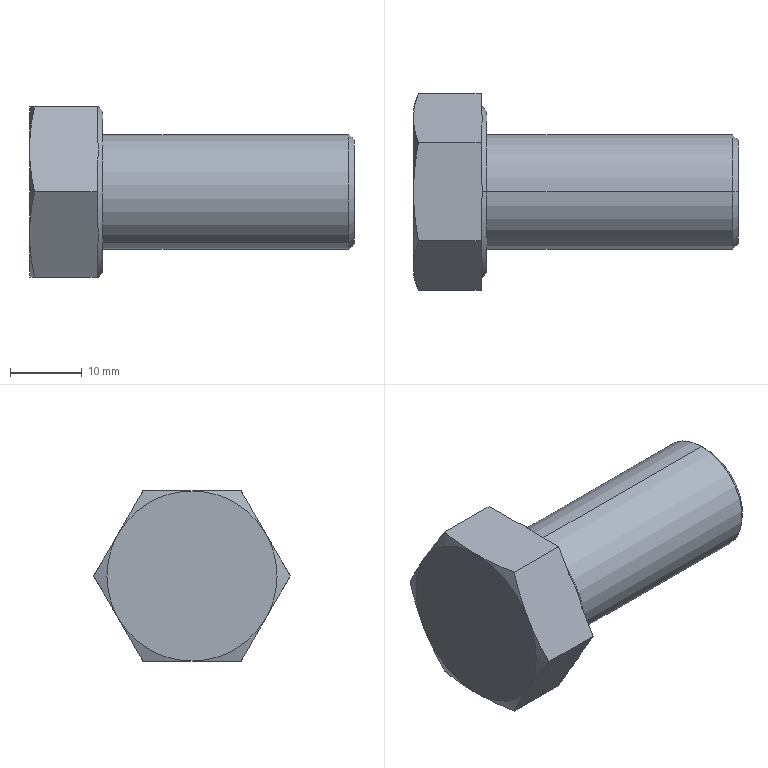Part | SolidWorks | 1 solid | 27 faces | box 45.18 x 27.332 x 23.67 mm | volume 11904 mm3 | plane 15 | cone 10 | cylinder 2 | commonest cylinder face diameters 16 x2
STEP:
#1=CARTESIAN_POINT('',(45.18,0.,-7.2));
#2=VERTEX_POINT('',#1);
#3=CARTESIAN_POINT('',(45.18,0.,7.2));
#4=VERTEX_POINT('',#3);
#5=CARTESIAN_POINT('',(45.18,0.,0.));
#6=DIRECTION('',(1.,0.,0.));
#7=DIRECTION('',(0.,0.,-1.));
#8=AXIS2_PLACEMENT_3D('',#5,#6,#7);
#9=CIRCLE('',#8,7.2);
#10=EDGE_CURVE('',#2,#4,#9,.T.);
#11=ORIENTED_EDGE('',*,*,#10,.F.);
#12=CARTESIAN_POINT('',(44.38,0.,-8.));
#13=VERTEX_POINT('',#12);
#14=CARTESIAN_POINT('',(45.18,0.,-7.2));
#15=DIRECTION('',(-0.7071,0.,-0.7071));
#16=VECTOR('',#15,1000.);
#17=LINE('',#14,#16);
#18=EDGE_CURVE('',#2,#13,#17,.T.);
#19=ORIENTED_EDGE('',*,*,#18,.T.);
#20=CARTESIAN_POINT('',(44.38,0.,8.));
#21=VERTEX_POINT('',#20);
#22=CARTESIAN_POINT('',(44.38,0.,0.));
#23=DIRECTION('',(-1.,0.,0.));
#24=DIRECTION('',(0.,0.,-1.));
#25=AXIS2_PLACEMENT_3D('',#22,#23,#24);
#26=CIRCLE('',#25,8.);
#27=EDGE_CURVE('',#21,#13,#26,.T.);
#28=ORIENTED_EDGE('',*,*,#27,.F.);
#29=CARTESIAN_POINT('',(45.18,0.,7.2));
#30=DIRECTION('',(-0.7071,0.,0.7071));
#31=VECTOR('',#30,1000.);
#32=LINE('',#29,#31);
#33=EDGE_CURVE('',#4,#21,#32,.T.);
#34=ORIENTED_EDGE('',*,*,#33,.F.);
#35=EDGE_LOOP('',(#11,#19,#28,#34));
#36=FACE_OUTER_BOUND('',#35,.T.);
#37=CARTESIAN_POINT('',(45.18,0.,0.));
#38=DIRECTION('',(-1.,0.,0.));
#39=DIRECTION('',(0.,0.,1.));
#40=AXIS2_PLACEMENT_3D('',#37,#38,#39);
#41=CONICAL_SURFACE('',#40,7.2,0.7854);
#42=ADVANCED_FACE('',(#36),#41,.T.);
#43=ORIENTED_EDGE('',*,*,#27,.T.);
#44=CARTESIAN_POINT('',(10.18,0.,-8.));
#45=VERTEX_POINT('',#44);
#46=CARTESIAN_POINT('',(45.18,0.,-8.));
#47=DIRECTION('',(-1.,0.,0.));
#48=VECTOR('',#47,1000.);
#49=LINE('',#46,#48);
#50=EDGE_CURVE('',#13,#45,#49,.T.);
#51=ORIENTED_EDGE('',*,*,#50,.T.);
#52=CARTESIAN_POINT('',(10.18,0.,8.));
#53=VERTEX_POINT('',#52);
#54=CARTESIAN_POINT('',(10.18,0.,0.));
#55=DIRECTION('',(1.,0.,0.));
#56=DIRECTION('',(0.,0.,1.));
#57=AXIS2_PLACEMENT_3D('',#54,#55,#56);
#58=CIRCLE('',#57,8.);
#59=EDGE_CURVE('',#45,#53,#58,.T.);
#60=ORIENTED_EDGE('',*,*,#59,.T.);
#61=CARTESIAN_POINT('',(45.18,0.,8.));
#62=DIRECTION('',(-1.,0.,0.));
#63=VECTOR('',#62,1000.);
#64=LINE('',#61,#63);
#65=EDGE_CURVE('',#21,#53,#64,.T.);
#66=ORIENTED_EDGE('',*,*,#65,.F.);
#67=EDGE_LOOP('',(#43,#51,#60,#66));
#68=FACE_OUTER_BOUND('',#67,.T.);
#69=CARTESIAN_POINT('',(45.18,0.,0.));
#70=DIRECTION('',(-1.,0.,0.));
#71=DIRECTION('',(0.,0.,1.));
#72=AXIS2_PLACEMENT_3D('',#69,#70,#71);
#73=CYLINDRICAL_SURFACE('',#72,8.);
#74=ADVANCED_FACE('',(#68),#73,.T.);
#75=CARTESIAN_POINT('',(10.18,0.,11.245));
#76=VERTEX_POINT('',#75);
#77=CARTESIAN_POINT('',(10.18,0.,-11.245));
#78=VERTEX_POINT('',#77);
#79=CARTESIAN_POINT('',(10.18,0.,0.));
#80=DIRECTION('',(-1.,0.,0.));
#81=DIRECTION('',(0.,0.,1.));
#82=AXIS2_PLACEMENT_3D('',#79,#80,#81);
#83=CIRCLE('',#82,11.245);
#84=EDGE_CURVE('',#76,#78,#83,.T.);
#85=ORIENTED_EDGE('',*,*,#84,.T.);
#86=CARTESIAN_POINT('',(9.59,0.,-11.835));
#87=VERTEX_POINT('',#86);
#88=CARTESIAN_POINT('',(9.38,0.,-12.045));
#89=DIRECTION('',(-0.7071,0.,-0.7071));
#90=VECTOR('',#89,1000.);
#91=LINE('',#88,#90);
#92=EDGE_CURVE('',#78,#87,#91,.T.);
#93=ORIENTED_EDGE('',*,*,#92,.T.);
#94=CARTESIAN_POINT('',(9.38,2.239,-11.835));
#95=VERTEX_POINT('',#94);
#96=CARTESIAN_POINT('',(9.59,0.,-11.835));
#97=CARTESIAN_POINT('',(9.59,0.3738,-11.835));
#98=CARTESIAN_POINT('',(9.572,0.7475,-11.835));
#99=CARTESIAN_POINT('',(9.502,1.495,-11.835));
#100=CARTESIAN_POINT('',(9.449,1.87,-11.835));
#101=CARTESIAN_POINT('',(9.38,2.239,-11.835));
#102=B_SPLINE_CURVE_WITH_KNOTS('',3,(#96,#97,#98,#99,#100,#101),.UNSPECIFIED.,.F.,.F.,(4,2,4),(0.00667,0.007787,0.008904),.UNSPECIFIED.);
#103=EDGE_CURVE('',#87,#95,#102,.T.);
#104=ORIENTED_EDGE('',*,*,#103,.T.);
#105=CARTESIAN_POINT('',(9.38,9.13,-7.857));
#106=VERTEX_POINT('',#105);
#107=CARTESIAN_POINT('',(9.38,0.,0.));
#108=DIRECTION('',(-1.,0.,0.));
#109=DIRECTION('',(0.,0.,1.));
#110=AXIS2_PLACEMENT_3D('',#107,#108,#109);
#111=CIRCLE('',#110,12.045);
#112=EDGE_CURVE('',#106,#95,#111,.T.);
#113=ORIENTED_EDGE('',*,*,#112,.F.);
#114=CARTESIAN_POINT('',(9.38,11.369,-3.978));
#115=VERTEX_POINT('',#114);
#116=CARTESIAN_POINT('',(9.38,9.13,-7.857));
#117=CARTESIAN_POINT('',(9.518,9.501,-7.214));
#118=CARTESIAN_POINT('',(9.59,9.873,-6.569));
#119=CARTESIAN_POINT('',(9.59,10.621,-5.274));
#120=CARTESIAN_POINT('',(9.518,10.998,-4.621));
#121=CARTESIAN_POINT('',(9.38,11.369,-3.978));
#122=B_SPLINE_CURVE_WITH_KNOTS('',3,(#116,#117,#118,#119,#120,#121),.UNSPECIFIED.,.F.,.F.,(4,2,4),(0.000001082,0.002242,0.004483),.UNSPECIFIED.);
#123=EDGE_CURVE('',#106,#115,#122,.T.);
#124=ORIENTED_EDGE('',*,*,#123,.T.);
#125=CARTESIAN_POINT('',(9.38,11.369,3.978));
#126=VERTEX_POINT('',#125);
#127=CARTESIAN_POINT('',(9.38,0.,0.));
#128=DIRECTION('',(-1.,0.,0.));
#129=DIRECTION('',(0.,0.,1.));
#130=AXIS2_PLACEMENT_3D('',#127,#128,#129);
#131=CIRCLE('',#130,12.045);
#132=EDGE_CURVE('',#126,#115,#131,.T.);
#133=ORIENTED_EDGE('',*,*,#132,.F.);
#134=CARTESIAN_POINT('',(9.38,9.13,7.857));
#135=VERTEX_POINT('',#134);
#136=CARTESIAN_POINT('',(9.38,11.369,3.978));
#137=CARTESIAN_POINT('',(9.518,10.998,4.621));
#138=CARTESIAN_POINT('',(9.59,10.626,5.266));
#139=CARTESIAN_POINT('',(9.59,9.878,6.561));
#140=CARTESIAN_POINT('',(9.518,9.501,7.214));
#141=CARTESIAN_POINT('',(9.38,9.13,7.857));
#142=B_SPLINE_CURVE_WITH_KNOTS('',3,(#136,#137,#138,#139,#140,#141),.UNSPECIFIED.,.F.,.F.,(4,2,4),(0.000001082,0.002242,0.004483),.UNSPECIFIED.);
#143=EDGE_CURVE('',#126,#135,#142,.T.);
#144=ORIENTED_EDGE('',*,*,#143,.T.);
#145=CARTESIAN_POINT('',(9.38,2.239,11.835));
#146=VERTEX_POINT('',#145);
#147=CARTESIAN_POINT('',(9.38,0.,0.));
#148=DIRECTION('',(-1.,0.,0.));
#149=DIRECTION('',(0.,0.,1.));
#150=AXIS2_PLACEMENT_3D('',#147,#148,#149);
#151=CIRCLE('',#150,12.045);
#152=EDGE_CURVE('',#146,#135,#151,.T.);
#153=ORIENTED_EDGE('',*,*,#152,.F.);
#154=CARTESIAN_POINT('',(9.59,0.,11.835));
#155=VERTEX_POINT('',#154);
#156=CARTESIAN_POINT('',(9.38,2.239,11.835));
#157=CARTESIAN_POINT('',(9.449,1.87,11.835));
#158=CARTESIAN_POINT('',(9.502,1.495,11.835));
#159=CARTESIAN_POINT('',(9.572,0.7475,11.835));
#160=CARTESIAN_POINT('',(9.59,0.3738,11.835));
#161=CARTESIAN_POINT('',(9.59,0.,11.835));
#162=B_SPLINE_CURVE_WITH_KNOTS('',3,(#156,#157,#158,#159,#160,#161),.UNSPECIFIED.,.F.,.F.,(4,2,4),(0.004938,0.006055,0.007171),.UNSPECIFIED.);
#163=EDGE_CURVE('',#146,#155,#162,.T.);
#164=ORIENTED_EDGE('',*,*,#163,.T.);
#165=CARTESIAN_POINT('',(9.38,0.,12.045));
#166=DIRECTION('',(-0.7071,0.,0.7071));
#167=VECTOR('',#166,1000.);
#168=LINE('',#165,#167);
#169=EDGE_CURVE('',#76,#155,#168,.T.);
#170=ORIENTED_EDGE('',*,*,#169,.F.);
#171=EDGE_LOOP('',(#85,#93,#104,#113,#124,#133,#144,#153,#164,#170));
#172=FACE_OUTER_BOUND('',#171,.T.);
#173=CARTESIAN_POINT('',(9.38,0.,0.));
#174=DIRECTION('',(-1.,0.,0.));
#175=DIRECTION('',(0.,0.,1.));
#176=AXIS2_PLACEMENT_3D('',#173,#174,#175);
#177=CONICAL_SURFACE('',#176,12.045,0.7854);
#178=ADVANCED_FACE('',(#172),#177,.T.);
#179=ORIENTED_EDGE('',*,*,#84,.F.);
#180=CARTESIAN_POINT('',(10.18,0.,0.));
#181=DIRECTION('',(-1.,0.,0.));
#182=DIRECTION('',(0.,0.,1.));
#183=AXIS2_PLACEMENT_3D('',#180,#181,#182);
#184=CIRCLE('',#183,11.245);
#185=EDGE_CURVE('',#78,#76,#184,.T.);
#186=ORIENTED_EDGE('',*,*,#185,.F.);
#187=EDGE_LOOP('',(#179,#186));
#188=FACE_OUTER_BOUND('',#187,.T.);
#189=CARTESIAN_POINT('',(10.18,0.,0.));
#190=DIRECTION('',(1.,0.,0.));
#191=DIRECTION('',(0.,0.,1.));
#192=AXIS2_PLACEMENT_3D('',#189,#190,#191);
#193=CIRCLE('',#192,8.);
#194=EDGE_CURVE('',#53,#45,#193,.T.);
#195=ORIENTED_EDGE('',*,*,#194,.F.);
#196=ORIENTED_EDGE('',*,*,#59,.F.);
#197=EDGE_LOOP('',(#195,#196));
#198=FACE_BOUND('',#197,.T.);
#199=CARTESIAN_POINT('',(10.18,-20.499,11.835));
#200=DIRECTION('',(-1.,0.,0.));
#201=DIRECTION('',(0.,0.,1.));
#202=AXIS2_PLACEMENT_3D('',#199,#200,#201);
#203=PLANE('',#202);
#204=ADVANCED_FACE('',(#188,#198),#203,.F.);
#205=CARTESIAN_POINT('',(0.6664,-6.833,-11.835));
#206=VERTEX_POINT('',#205);
#207=CARTESIAN_POINT('',(0.,-10.249,-5.917));
#208=VERTEX_POINT('',#207);
#209=CARTESIAN_POINT('',(0.6664,-6.833,-11.835));
#210=CARTESIAN_POINT('',(0.4591,-7.402,-10.849));
#211=CARTESIAN_POINT('',(0.2909,-7.972,-9.862));
#212=CARTESIAN_POINT('',(0.06093,-9.111,-7.89));
#213=CARTESIAN_POINT('',(0.,-9.68,-6.904));
#214=CARTESIAN_POINT('',(0.,-10.249,-5.917));
#215=B_SPLINE_CURVE_WITH_KNOTS('',3,(#209,#210,#211,#212,#213,#214),.UNSPECIFIED.,.F.,.F.,(4,2,4),(0.000000231,0.003417,0.006833),.UNSPECIFIED.);
#216=EDGE_CURVE('',#206,#208,#215,.T.);
#217=ORIENTED_EDGE('',*,*,#216,.F.);
#218=CARTESIAN_POINT('',(9.38,-6.833,-11.835));
#219=VERTEX_POINT('',#218);
#220=CARTESIAN_POINT('',(10.18,-6.833,-11.835));
#221=DIRECTION('',(-1.,0.,0.));
#222=VECTOR('',#221,1000.);
#223=LINE('',#220,#222);
#224=EDGE_CURVE('',#219,#206,#223,.T.);
#225=ORIENTED_EDGE('',*,*,#224,.F.);
#226=CARTESIAN_POINT('',(9.38,-9.13,-7.857));
#227=VERTEX_POINT('',#226);
#228=CARTESIAN_POINT('',(9.38,-13.666,0.));
#229=DIRECTION('',(0.,0.5,-0.866));
#230=VECTOR('',#229,1000.);
#231=LINE('',#228,#230);
#232=EDGE_CURVE('',#227,#219,#231,.T.);
#233=ORIENTED_EDGE('',*,*,#232,.F.);
#234=CARTESIAN_POINT('',(9.38,-11.369,-3.978));
#235=VERTEX_POINT('',#234);
#236=CARTESIAN_POINT('',(9.38,-11.369,-3.978));
#237=CARTESIAN_POINT('',(9.518,-10.998,-4.621));
#238=CARTESIAN_POINT('',(9.59,-10.626,-5.266));
#239=CARTESIAN_POINT('',(9.59,-9.878,-6.561));
#240=CARTESIAN_POINT('',(9.518,-9.501,-7.214));
#241=CARTESIAN_POINT('',(9.38,-9.13,-7.857));
#242=B_SPLINE_CURVE_WITH_KNOTS('',3,(#236,#237,#238,#239,#240,#241),.UNSPECIFIED.,.F.,.F.,(4,2,4),(0.000001082,0.002242,0.004483),.UNSPECIFIED.);
#243=EDGE_CURVE('',#235,#227,#242,.T.);
#244=ORIENTED_EDGE('',*,*,#243,.F.);
#245=CARTESIAN_POINT('',(9.38,-13.666,0.));
#246=VERTEX_POINT('',#245);
#247=CARTESIAN_POINT('',(9.38,-13.666,0.));
#248=DIRECTION('',(0.,0.5,-0.866));
#249=VECTOR('',#248,1000.);
#250=LINE('',#247,#249);
#251=EDGE_CURVE('',#246,#235,#250,.T.);
#252=ORIENTED_EDGE('',*,*,#251,.F.);
#253=CARTESIAN_POINT('',(0.6664,-13.666,0.));
#254=VERTEX_POINT('',#253);
#255=CARTESIAN_POINT('',(10.18,-13.666,0.));
#256=DIRECTION('',(-1.,0.,0.));
#257=VECTOR('',#256,1000.);
#258=LINE('',#255,#257);
#259=EDGE_CURVE('',#246,#254,#258,.T.);
#260=ORIENTED_EDGE('',*,*,#259,.T.);
#261=CARTESIAN_POINT('',(0.,-10.249,-5.917));
#262=CARTESIAN_POINT('',(0.,-10.819,-4.931));
#263=CARTESIAN_POINT('',(0.06093,-11.388,-3.945));
#264=CARTESIAN_POINT('',(0.2909,-12.527,-1.972));
#265=CARTESIAN_POINT('',(0.4591,-13.096,-0.9862));
#266=CARTESIAN_POINT('',(0.6664,-13.666,0.));
#267=B_SPLINE_CURVE_WITH_KNOTS('',3,(#261,#262,#263,#264,#265,#266),.UNSPECIFIED.,.F.,.F.,(4,2,4),(0.006833,0.01025,0.01367),.UNSPECIFIED.);
#268=EDGE_CURVE('',#208,#254,#267,.T.);
#269=ORIENTED_EDGE('',*,*,#268,.F.);
#270=EDGE_LOOP('',(#217,#225,#233,#244,#252,#260,#269));
#271=FACE_OUTER_BOUND('',#270,.T.);
#272=CARTESIAN_POINT('',(10.18,-13.666,0.));
#273=DIRECTION('',(0.,0.866,0.5));
#274=DIRECTION('',(0.,-0.5,0.866));
#275=AXIS2_PLACEMENT_3D('',#272,#273,#274);
#276=PLANE('',#275);
#277=ADVANCED_FACE('',(#271),#276,.F.);
#278=CARTESIAN_POINT('',(0.6664,6.833,-11.835));
#279=VERTEX_POINT('',#278);
#280=CARTESIAN_POINT('',(0.,0.,-11.835));
#281=VERTEX_POINT('',#280);
#282=CARTESIAN_POINT('',(0.6664,6.833,-11.835));
#283=CARTESIAN_POINT('',(0.4597,5.697,-11.835));
#284=CARTESIAN_POINT('',(0.2913,4.559,-11.835));
#285=CARTESIAN_POINT('',(0.06117,2.281,-11.835));
#286=CARTESIAN_POINT('',(0.,1.141,-11.835));
#287=CARTESIAN_POINT('',(0.,0.,-11.835));
#288=B_SPLINE_CURVE_WITH_KNOTS('',3,(#282,#283,#284,#285,#286,#287),.UNSPECIFIED.,.F.,.F.,(4,2,4),(0.02464,0.02808,0.03153),.UNSPECIFIED.);
#289=EDGE_CURVE('',#279,#281,#288,.T.);
#290=ORIENTED_EDGE('',*,*,#289,.F.);
#291=CARTESIAN_POINT('',(9.38,6.833,-11.835));
#292=VERTEX_POINT('',#291);
#293=CARTESIAN_POINT('',(10.18,6.833,-11.835));
#294=DIRECTION('',(-1.,0.,0.));
#295=VECTOR('',#294,1000.);
#296=LINE('',#293,#295);
#297=EDGE_CURVE('',#292,#279,#296,.T.);
#298=ORIENTED_EDGE('',*,*,#297,.F.);
#299=CARTESIAN_POINT('',(9.38,-6.833,-11.835));
#300=DIRECTION('',(0.,1.,0.));
#301=VECTOR('',#300,1000.);
#302=LINE('',#299,#301);
#303=EDGE_CURVE('',#95,#292,#302,.T.);
#304=ORIENTED_EDGE('',*,*,#303,.F.);
#305=ORIENTED_EDGE('',*,*,#103,.F.);
#306=CARTESIAN_POINT('',(9.38,-2.239,-11.835));
#307=VERTEX_POINT('',#306);
#308=CARTESIAN_POINT('',(9.38,-2.239,-11.835));
#309=CARTESIAN_POINT('',(9.449,-1.871,-11.835));
#310=CARTESIAN_POINT('',(9.502,-1.495,-11.835));
#311=CARTESIAN_POINT('',(9.572,-0.7474,-11.835));
#312=CARTESIAN_POINT('',(9.59,-0.3736,-11.835));
#313=CARTESIAN_POINT('',(9.59,0.,-11.835));
#314=B_SPLINE_CURVE_WITH_KNOTS('',3,(#308,#309,#310,#311,#312,#313),.UNSPECIFIED.,.F.,.F.,(4,2,4),(0.004436,0.005553,0.00667),.UNSPECIFIED.);
#315=EDGE_CURVE('',#307,#87,#314,.T.);
#316=ORIENTED_EDGE('',*,*,#315,.F.);
#317=CARTESIAN_POINT('',(9.38,-6.833,-11.835));
#318=DIRECTION('',(0.,1.,0.));
#319=VECTOR('',#318,1000.);
#320=LINE('',#317,#319);
#321=EDGE_CURVE('',#219,#307,#320,.T.);
#322=ORIENTED_EDGE('',*,*,#321,.F.);
#323=ORIENTED_EDGE('',*,*,#224,.T.);
#324=CARTESIAN_POINT('',(0.,0.,-11.835));
#325=CARTESIAN_POINT('',(0.,-1.138,-11.835));
#326=CARTESIAN_POINT('',(0.06084,-2.277,-11.835));
#327=CARTESIAN_POINT('',(0.2911,-4.558,-11.835));
#328=CARTESIAN_POINT('',(0.4605,-5.702,-11.835));
#329=CARTESIAN_POINT('',(0.6664,-6.833,-11.835));
#330=B_SPLINE_CURVE_WITH_KNOTS('',3,(#324,#325,#326,#327,#328,#329),.UNSPECIFIED.,.F.,.F.,(4,2,4),(0.03153,0.03496,0.0384),.UNSPECIFIED.);
#331=EDGE_CURVE('',#281,#206,#330,.T.);
#332=ORIENTED_EDGE('',*,*,#331,.F.);
#333=EDGE_LOOP('',(#290,#298,#304,#305,#316,#322,#323,#332));
#334=FACE_OUTER_BOUND('',#333,.T.);
#335=CARTESIAN_POINT('',(10.18,-6.833,-11.835));
#336=DIRECTION('',(0.,0.,1.));
#337=DIRECTION('',(0.,-1.,0.));
#338=AXIS2_PLACEMENT_3D('',#335,#336,#337);
#339=PLANE('',#338);
#340=ADVANCED_FACE('',(#334),#339,.F.);
#341=CARTESIAN_POINT('',(0.6664,13.666,0.));
#342=VERTEX_POINT('',#341);
#343=CARTESIAN_POINT('',(0.,10.249,-5.917));
#344=VERTEX_POINT('',#343);
#345=CARTESIAN_POINT('',(0.6664,13.666,0.));
#346=CARTESIAN_POINT('',(0.4591,13.096,-0.9863));
#347=CARTESIAN_POINT('',(0.2909,12.527,-1.972));
#348=CARTESIAN_POINT('',(0.06093,11.388,-3.945));
#349=CARTESIAN_POINT('',(0.,10.819,-4.931));
#350=CARTESIAN_POINT('',(0.,10.249,-5.917));
#351=B_SPLINE_CURVE_WITH_KNOTS('',3,(#345,#346,#347,#348,#349,#350),.UNSPECIFIED.,.F.,.F.,(4,2,4),(0.000000231,0.003417,0.006833),.UNSPECIFIED.);
#352=EDGE_CURVE('',#342,#344,#351,.T.);
#353=ORIENTED_EDGE('',*,*,#352,.F.);
#354=CARTESIAN_POINT('',(9.38,13.666,0.));
#355=VERTEX_POINT('',#354);
#356=CARTESIAN_POINT('',(10.18,13.666,0.));
#357=DIRECTION('',(-1.,0.,0.));
#358=VECTOR('',#357,1000.);
#359=LINE('',#356,#358);
#360=EDGE_CURVE('',#355,#342,#359,.T.);
#361=ORIENTED_EDGE('',*,*,#360,.F.);
#362=CARTESIAN_POINT('',(9.38,6.833,-11.835));
#363=DIRECTION('',(0.,0.5,0.866));
#364=VECTOR('',#363,1000.);
#365=LINE('',#362,#364);
#366=EDGE_CURVE('',#115,#355,#365,.T.);
#367=ORIENTED_EDGE('',*,*,#366,.F.);
#368=ORIENTED_EDGE('',*,*,#123,.F.);
#369=CARTESIAN_POINT('',(9.38,6.833,-11.835));
#370=DIRECTION('',(0.,0.5,0.866));
#371=VECTOR('',#370,1000.);
#372=LINE('',#369,#371);
#373=EDGE_CURVE('',#292,#106,#372,.T.);
#374=ORIENTED_EDGE('',*,*,#373,.F.);
#375=ORIENTED_EDGE('',*,*,#297,.T.);
#376=CARTESIAN_POINT('',(0.,10.249,-5.917));
#377=CARTESIAN_POINT('',(0.,9.68,-6.904));
#378=CARTESIAN_POINT('',(0.06093,9.111,-7.89));
#379=CARTESIAN_POINT('',(0.2909,7.972,-9.862));
#380=CARTESIAN_POINT('',(0.4591,7.402,-10.849));
#381=CARTESIAN_POINT('',(0.6664,6.833,-11.835));
#382=B_SPLINE_CURVE_WITH_KNOTS('',3,(#376,#377,#378,#379,#380,#381),.UNSPECIFIED.,.F.,.F.,(4,2,4),(0.006833,0.01025,0.01367),.UNSPECIFIED.);
#383=EDGE_CURVE('',#344,#279,#382,.T.);
#384=ORIENTED_EDGE('',*,*,#383,.F.);
#385=EDGE_LOOP('',(#353,#361,#367,#368,#374,#375,#384));
#386=FACE_OUTER_BOUND('',#385,.T.);
#387=CARTESIAN_POINT('',(10.18,6.833,-11.835));
#388=DIRECTION('',(0.,-0.866,0.5));
#389=DIRECTION('',(0.,-0.5,-0.866));
#390=AXIS2_PLACEMENT_3D('',#387,#388,#389);
#391=PLANE('',#390);
#392=ADVANCED_FACE('',(#386),#391,.F.);
#393=CARTESIAN_POINT('',(0.6664,6.833,11.835));
#394=VERTEX_POINT('',#393);
#395=CARTESIAN_POINT('',(0.,10.249,5.917));
#396=VERTEX_POINT('',#395);
#397=CARTESIAN_POINT('',(0.6664,6.833,11.835));
#398=CARTESIAN_POINT('',(0.4591,7.402,10.849));
#399=CARTESIAN_POINT('',(0.2909,7.972,9.863));
#400=CARTESIAN_POINT('',(0.06093,9.111,7.89));
#401=CARTESIAN_POINT('',(0.,9.68,6.904));
#402=CARTESIAN_POINT('',(0.,10.249,5.917));
#403=B_SPLINE_CURVE_WITH_KNOTS('',3,(#397,#398,#399,#400,#401,#402),.UNSPECIFIED.,.F.,.F.,(4,2,4),(0.000000231,0.003417,0.006833),.UNSPECIFIED.);
#404=EDGE_CURVE('',#394,#396,#403,.T.);
#405=ORIENTED_EDGE('',*,*,#404,.F.);
#406=CARTESIAN_POINT('',(9.38,6.833,11.835));
#407=VERTEX_POINT('',#406);
#408=CARTESIAN_POINT('',(10.18,6.833,11.835));
#409=DIRECTION('',(-1.,0.,0.));
#410=VECTOR('',#409,1000.);
#411=LINE('',#408,#410);
#412=EDGE_CURVE('',#407,#394,#411,.T.);
#413=ORIENTED_EDGE('',*,*,#412,.F.);
#414=CARTESIAN_POINT('',(9.38,13.666,0.));
#415=DIRECTION('',(0.,-0.5,0.866));
#416=VECTOR('',#415,1000.);
#417=LINE('',#414,#416);
#418=EDGE_CURVE('',#135,#407,#417,.T.);
#419=ORIENTED_EDGE('',*,*,#418,.F.);
#420=ORIENTED_EDGE('',*,*,#143,.F.);
#421=CARTESIAN_POINT('',(9.38,13.666,0.));
#422=DIRECTION('',(0.,-0.5,0.866));
#423=VECTOR('',#422,1000.);
#424=LINE('',#421,#423);
#425=EDGE_CURVE('',#355,#126,#424,.T.);
#426=ORIENTED_EDGE('',*,*,#425,.F.);
#427=ORIENTED_EDGE('',*,*,#360,.T.);
#428=CARTESIAN_POINT('',(0.,10.249,5.917));
#429=CARTESIAN_POINT('',(0.,10.819,4.931));
#430=CARTESIAN_POINT('',(0.06093,11.388,3.945));
#431=CARTESIAN_POINT('',(0.2909,12.527,1.972));
#432=CARTESIAN_POINT('',(0.4591,13.096,0.9862));
#433=CARTESIAN_POINT('',(0.6664,13.666,0.));
#434=B_SPLINE_CURVE_WITH_KNOTS('',3,(#428,#429,#430,#431,#432,#433),.UNSPECIFIED.,.F.,.F.,(4,2,4),(0.006833,0.01025,0.01367),.UNSPECIFIED.);
#435=EDGE_CURVE('',#396,#342,#434,.T.);
#436=ORIENTED_EDGE('',*,*,#435,.F.);
#437=EDGE_LOOP('',(#405,#413,#419,#420,#426,#427,#436));
#438=FACE_OUTER_BOUND('',#437,.T.);
#439=CARTESIAN_POINT('',(10.18,13.666,0.));
#440=DIRECTION('',(0.,-0.866,-0.5));
#441=DIRECTION('',(0.,0.5,-0.866));
#442=AXIS2_PLACEMENT_3D('',#439,#440,#441);
#443=PLANE('',#442);
#444=ADVANCED_FACE('',(#438),#443,.F.);
#445=CARTESIAN_POINT('',(0.6664,-6.833,11.835));
#446=VERTEX_POINT('',#445);
#447=CARTESIAN_POINT('',(0.,0.,11.835));
#448=VERTEX_POINT('',#447);
#449=CARTESIAN_POINT('',(0.6664,-6.833,11.835));
#450=CARTESIAN_POINT('',(0.4605,-5.702,11.835));
#451=CARTESIAN_POINT('',(0.2911,-4.558,11.835));
#452=CARTESIAN_POINT('',(0.06084,-2.277,11.835));
#453=CARTESIAN_POINT('',(0.,-1.138,11.835));
#454=CARTESIAN_POINT('',(0.,0.,11.835));
#455=B_SPLINE_CURVE_WITH_KNOTS('',3,(#449,#450,#451,#452,#453,#454),.UNSPECIFIED.,.F.,.F.,(4,2,4),(0.01162,0.01507,0.01851),.UNSPECIFIED.);
#456=EDGE_CURVE('',#446,#448,#455,.T.);
#457=ORIENTED_EDGE('',*,*,#456,.F.);
#458=CARTESIAN_POINT('',(9.38,-6.833,11.835));
#459=VERTEX_POINT('',#458);
#460=CARTESIAN_POINT('',(10.18,-6.833,11.835));
#461=DIRECTION('',(-1.,0.,0.));
#462=VECTOR('',#461,1000.);
#463=LINE('',#460,#462);
#464=EDGE_CURVE('',#459,#446,#463,.T.);
#465=ORIENTED_EDGE('',*,*,#464,.F.);
#466=CARTESIAN_POINT('',(9.38,-2.239,11.835));
#467=VERTEX_POINT('',#466);
#468=CARTESIAN_POINT('',(9.38,6.833,11.835));
#469=DIRECTION('',(0.,-1.,0.));
#470=VECTOR('',#469,1000.);
#471=LINE('',#468,#470);
#472=EDGE_CURVE('',#467,#459,#471,.T.);
#473=ORIENTED_EDGE('',*,*,#472,.F.);
#474=CARTESIAN_POINT('',(9.59,0.,11.835));
#475=CARTESIAN_POINT('',(9.59,-0.3736,11.835));
#476=CARTESIAN_POINT('',(9.572,-0.7474,11.835));
#477=CARTESIAN_POINT('',(9.502,-1.495,11.835));
#478=CARTESIAN_POINT('',(9.449,-1.871,11.835));
#479=CARTESIAN_POINT('',(9.38,-2.239,11.835));
#480=B_SPLINE_CURVE_WITH_KNOTS('',3,(#474,#475,#476,#477,#478,#479),.UNSPECIFIED.,.F.,.F.,(4,2,4),(0.007171,0.008287,0.009403),.UNSPECIFIED.);
#481=EDGE_CURVE('',#155,#467,#480,.T.);
#482=ORIENTED_EDGE('',*,*,#481,.F.);
#483=ORIENTED_EDGE('',*,*,#163,.F.);
#484=CARTESIAN_POINT('',(9.38,6.833,11.835));
#485=DIRECTION('',(0.,-1.,0.));
#486=VECTOR('',#485,1000.);
#487=LINE('',#484,#486);
#488=EDGE_CURVE('',#407,#146,#487,.T.);
#489=ORIENTED_EDGE('',*,*,#488,.F.);
#490=ORIENTED_EDGE('',*,*,#412,.T.);
#491=CARTESIAN_POINT('',(0.,0.,11.835));
#492=CARTESIAN_POINT('',(0.,1.141,11.835));
#493=CARTESIAN_POINT('',(0.06117,2.281,11.835));
#494=CARTESIAN_POINT('',(0.2913,4.559,11.835));
#495=CARTESIAN_POINT('',(0.4597,5.697,11.835));
#496=CARTESIAN_POINT('',(0.6664,6.833,11.835));
#497=B_SPLINE_CURVE_WITH_KNOTS('',3,(#491,#492,#493,#494,#495,#496),.UNSPECIFIED.,.F.,.F.,(4,2,4),(0.01851,0.02196,0.02542),.UNSPECIFIED.);
#498=EDGE_CURVE('',#448,#394,#497,.T.);
#499=ORIENTED_EDGE('',*,*,#498,.F.);
#500=EDGE_LOOP('',(#457,#465,#473,#482,#483,#489,#490,#499));
#501=FACE_OUTER_BOUND('',#500,.T.);
#502=CARTESIAN_POINT('',(10.18,6.833,11.835));
#503=DIRECTION('',(0.,0.,-1.));
#504=DIRECTION('',(-1.,0.,0.));
#505=AXIS2_PLACEMENT_3D('',#502,#503,#504);
#506=PLANE('',#505);
#507=ADVANCED_FACE('',(#501),#506,.F.);
#508=CARTESIAN_POINT('',(0.,-10.249,5.918));
#509=VERTEX_POINT('',#508);
#510=CARTESIAN_POINT('',(0.6664,-13.666,0.));
#511=CARTESIAN_POINT('',(0.4591,-13.096,0.9863));
#512=CARTESIAN_POINT('',(0.2909,-12.527,1.973));
#513=CARTESIAN_POINT('',(0.06093,-11.388,3.945));
#514=CARTESIAN_POINT('',(0.,-10.819,4.931));
#515=CARTESIAN_POINT('',(0.,-10.249,5.918));
#516=B_SPLINE_CURVE_WITH_KNOTS('',3,(#510,#511,#512,#513,#514,#515),.UNSPECIFIED.,.F.,.F.,(4,2,4),(0.000000231,0.003417,0.006833),.UNSPECIFIED.);
#517=EDGE_CURVE('',#254,#509,#516,.T.);
#518=ORIENTED_EDGE('',*,*,#517,.F.);
#519=ORIENTED_EDGE('',*,*,#259,.F.);
#520=CARTESIAN_POINT('',(9.38,-11.369,3.978));
#521=VERTEX_POINT('',#520);
#522=CARTESIAN_POINT('',(9.38,-6.833,11.835));
#523=DIRECTION('',(0.,-0.5,-0.866));
#524=VECTOR('',#523,1000.);
#525=LINE('',#522,#524);
#526=EDGE_CURVE('',#521,#246,#525,.T.);
#527=ORIENTED_EDGE('',*,*,#526,.F.);
#528=CARTESIAN_POINT('',(9.38,-9.13,7.857));
#529=VERTEX_POINT('',#528);
#530=CARTESIAN_POINT('',(9.38,-9.13,7.857));
#531=CARTESIAN_POINT('',(9.518,-9.501,7.214));
#532=CARTESIAN_POINT('',(9.59,-9.873,6.569));
#533=CARTESIAN_POINT('',(9.59,-10.621,5.274));
#534=CARTESIAN_POINT('',(9.518,-10.998,4.621));
#535=CARTESIAN_POINT('',(9.38,-11.369,3.978));
#536=B_SPLINE_CURVE_WITH_KNOTS('',3,(#530,#531,#532,#533,#534,#535),.UNSPECIFIED.,.F.,.F.,(4,2,4),(0.000001082,0.002242,0.004483),.UNSPECIFIED.);
#537=EDGE_CURVE('',#529,#521,#536,.T.);
#538=ORIENTED_EDGE('',*,*,#537,.F.);
#539=CARTESIAN_POINT('',(9.38,-6.833,11.835));
#540=DIRECTION('',(0.,-0.5,-0.866));
#541=VECTOR('',#540,1000.);
#542=LINE('',#539,#541);
#543=EDGE_CURVE('',#459,#529,#542,.T.);
#544=ORIENTED_EDGE('',*,*,#543,.F.);
#545=ORIENTED_EDGE('',*,*,#464,.T.);
#546=CARTESIAN_POINT('',(0.,-10.249,5.918));
#547=CARTESIAN_POINT('',(0.,-9.68,6.904));
#548=CARTESIAN_POINT('',(0.06093,-9.111,7.89));
#549=CARTESIAN_POINT('',(0.2909,-7.972,9.863));
#550=CARTESIAN_POINT('',(0.4591,-7.402,10.849));
#551=CARTESIAN_POINT('',(0.6664,-6.833,11.835));
#552=B_SPLINE_CURVE_WITH_KNOTS('',3,(#546,#547,#548,#549,#550,#551),.UNSPECIFIED.,.F.,.F.,(4,2,4),(0.006833,0.01025,0.01367),.UNSPECIFIED.);
#553=EDGE_CURVE('',#509,#446,#552,.T.);
#554=ORIENTED_EDGE('',*,*,#553,.F.);
#555=EDGE_LOOP('',(#518,#519,#527,#538,#544,#545,#554));
#556=FACE_OUTER_BOUND('',#555,.T.);
#557=CARTESIAN_POINT('',(10.18,-6.833,11.835));
#558=DIRECTION('',(0.,0.866,-0.5));
#559=DIRECTION('',(0.,0.5,0.866));
#560=AXIS2_PLACEMENT_3D('',#557,#558,#559);
#561=PLANE('',#560);
#562=ADVANCED_FACE('',(#556),#561,.F.);
#563=ORIENTED_EDGE('',*,*,#232,.T.);
#564=ORIENTED_EDGE('',*,*,#321,.T.);
#565=CARTESIAN_POINT('',(9.38,0.,0.));
#566=DIRECTION('',(-1.,0.,0.));
#567=DIRECTION('',(0.,0.,1.));
#568=AXIS2_PLACEMENT_3D('',#565,#566,#567);
#569=CIRCLE('',#568,12.045);
#570=EDGE_CURVE('',#307,#227,#569,.T.);
#571=ORIENTED_EDGE('',*,*,#570,.T.);
#572=EDGE_LOOP('',(#563,#564,#571));
#573=FACE_OUTER_BOUND('',#572,.T.);
#574=CARTESIAN_POINT('',(9.38,12.045,0.));
#575=DIRECTION('',(1.,0.,0.));
#576=DIRECTION('',(0.,0.,-1.));
#577=AXIS2_PLACEMENT_3D('',#574,#575,#576);
#578=PLANE('',#577);
#579=ADVANCED_FACE('',(#573),#578,.T.);
#580=ORIENTED_EDGE('',*,*,#303,.T.);
#581=ORIENTED_EDGE('',*,*,#373,.T.);
#582=ORIENTED_EDGE('',*,*,#112,.T.);
#583=EDGE_LOOP('',(#580,#581,#582));
#584=FACE_OUTER_BOUND('',#583,.T.);
#585=CARTESIAN_POINT('',(9.38,12.045,0.));
#586=DIRECTION('',(1.,0.,0.));
#587=DIRECTION('',(0.,0.,-1.));
#588=AXIS2_PLACEMENT_3D('',#585,#586,#587);
#589=PLANE('',#588);
#590=ADVANCED_FACE('',(#584),#589,.T.);
#591=ORIENTED_EDGE('',*,*,#366,.T.);
#592=ORIENTED_EDGE('',*,*,#425,.T.);
#593=ORIENTED_EDGE('',*,*,#132,.T.);
#594=EDGE_LOOP('',(#591,#592,#593));
#595=FACE_OUTER_BOUND('',#594,.T.);
#596=CARTESIAN_POINT('',(9.38,12.045,0.));
#597=DIRECTION('',(1.,0.,0.));
#598=DIRECTION('',(0.,0.,-1.));
#599=AXIS2_PLACEMENT_3D('',#596,#597,#598);
#600=PLANE('',#599);
#601=ADVANCED_FACE('',(#595),#600,.T.);
#602=ORIENTED_EDGE('',*,*,#418,.T.);
#603=ORIENTED_EDGE('',*,*,#488,.T.);
#604=ORIENTED_EDGE('',*,*,#152,.T.);
#605=EDGE_LOOP('',(#602,#603,#604));
#606=FACE_OUTER_BOUND('',#605,.T.);
#607=CARTESIAN_POINT('',(9.38,12.045,0.));
#608=DIRECTION('',(1.,0.,0.));
#609=DIRECTION('',(0.,0.,-1.));
#610=AXIS2_PLACEMENT_3D('',#607,#608,#609);
#611=PLANE('',#610);
#612=ADVANCED_FACE('',(#606),#611,.T.);
#613=ORIENTED_EDGE('',*,*,#472,.T.);
#614=ORIENTED_EDGE('',*,*,#543,.T.);
#615=CARTESIAN_POINT('',(9.38,0.,0.));
#616=DIRECTION('',(-1.,0.,0.));
#617=DIRECTION('',(0.,0.,1.));
#618=AXIS2_PLACEMENT_3D('',#615,#616,#617);
#619=CIRCLE('',#618,12.045);
#620=EDGE_CURVE('',#529,#467,#619,.T.);
#621=ORIENTED_EDGE('',*,*,#620,.T.);
#622=EDGE_LOOP('',(#613,#614,#621));
#623=FACE_OUTER_BOUND('',#622,.T.);
#624=CARTESIAN_POINT('',(9.38,12.045,0.));
#625=DIRECTION('',(1.,0.,0.));
#626=DIRECTION('',(0.,0.,-1.));
#627=AXIS2_PLACEMENT_3D('',#624,#625,#626);
#628=PLANE('',#627);
#629=ADVANCED_FACE('',(#623),#628,.T.);
#630=ORIENTED_EDGE('',*,*,#251,.T.);
#631=CARTESIAN_POINT('',(9.38,0.,0.));
#632=DIRECTION('',(-1.,0.,0.));
#633=DIRECTION('',(0.,0.,1.));
#634=AXIS2_PLACEMENT_3D('',#631,#632,#633);
#635=CIRCLE('',#634,12.045);
#636=EDGE_CURVE('',#235,#521,#635,.T.);
#637=ORIENTED_EDGE('',*,*,#636,.T.);
#638=ORIENTED_EDGE('',*,*,#526,.T.);
#639=EDGE_LOOP('',(#630,#637,#638));
#640=FACE_OUTER_BOUND('',#639,.T.);
#641=CARTESIAN_POINT('',(9.38,12.045,0.));
#642=DIRECTION('',(1.,0.,0.));
#643=DIRECTION('',(0.,0.,-1.));
#644=AXIS2_PLACEMENT_3D('',#641,#642,#643);
#645=PLANE('',#644);
#646=ADVANCED_FACE('',(#640),#645,.T.);
#647=ORIENTED_EDGE('',*,*,#92,.F.);
#648=ORIENTED_EDGE('',*,*,#185,.T.);
#649=ORIENTED_EDGE('',*,*,#169,.T.);
#650=ORIENTED_EDGE('',*,*,#481,.T.);
#651=ORIENTED_EDGE('',*,*,#620,.F.);
#652=ORIENTED_EDGE('',*,*,#537,.T.);
#653=ORIENTED_EDGE('',*,*,#636,.F.);
#654=ORIENTED_EDGE('',*,*,#243,.T.);
#655=ORIENTED_EDGE('',*,*,#570,.F.);
#656=ORIENTED_EDGE('',*,*,#315,.T.);
#657=EDGE_LOOP('',(#647,#648,#649,#650,#651,#652,#653,#654,#655,#656));
#658=FACE_OUTER_BOUND('',#657,.T.);
#659=CARTESIAN_POINT('',(9.38,0.,0.));
#660=DIRECTION('',(-1.,0.,0.));
#661=DIRECTION('',(0.,0.,1.));
#662=AXIS2_PLACEMENT_3D('',#659,#660,#661);
#663=CONICAL_SURFACE('',#662,12.045,0.7854);
#664=ADVANCED_FACE('',(#658),#663,.T.);
#665=ORIENTED_EDGE('',*,*,#456,.T.);
#666=CARTESIAN_POINT('',(0.,0.,0.));
#667=DIRECTION('',(-1.,0.,0.));
#668=DIRECTION('',(0.,0.,1.));
#669=AXIS2_PLACEMENT_3D('',#666,#667,#668);
#670=CIRCLE('',#669,11.835);
#671=EDGE_CURVE('',#509,#448,#670,.T.);
#672=ORIENTED_EDGE('',*,*,#671,.F.);
#673=ORIENTED_EDGE('',*,*,#553,.T.);
#674=EDGE_LOOP('',(#665,#672,#673));
#675=FACE_OUTER_BOUND('',#674,.T.);
#676=CARTESIAN_POINT('',(0.,0.,0.));
#677=DIRECTION('',(1.,0.,0.));
#678=DIRECTION('',(0.,0.,-1.));
#679=AXIS2_PLACEMENT_3D('',#676,#677,#678);
#680=CONICAL_SURFACE('',#679,11.835,1.222);
#681=ADVANCED_FACE('',(#675),#680,.T.);
#682=ORIENTED_EDGE('',*,*,#268,.T.);
#683=ORIENTED_EDGE('',*,*,#517,.T.);
#684=CARTESIAN_POINT('',(0.,0.,0.));
#685=DIRECTION('',(-1.,0.,0.));
#686=DIRECTION('',(0.,0.,1.));
#687=AXIS2_PLACEMENT_3D('',#684,#685,#686);
#688=CIRCLE('',#687,11.835);
#689=EDGE_CURVE('',#208,#509,#688,.T.);
#690=ORIENTED_EDGE('',*,*,#689,.F.);
#691=EDGE_LOOP('',(#682,#683,#690));
#692=FACE_OUTER_BOUND('',#691,.T.);
#693=CARTESIAN_POINT('',(0.,0.,0.));
#694=DIRECTION('',(1.,0.,0.));
#695=DIRECTION('',(0.,0.,-1.));
#696=AXIS2_PLACEMENT_3D('',#693,#694,#695);
#697=CONICAL_SURFACE('',#696,11.835,1.222);
#698=ADVANCED_FACE('',(#692),#697,.T.);
#699=ORIENTED_EDGE('',*,*,#331,.T.);
#700=ORIENTED_EDGE('',*,*,#216,.T.);
#701=CARTESIAN_POINT('',(0.,0.,0.));
#702=DIRECTION('',(-1.,0.,0.));
#703=DIRECTION('',(0.,0.,1.));
#704=AXIS2_PLACEMENT_3D('',#701,#702,#703);
#705=CIRCLE('',#704,11.835);
#706=EDGE_CURVE('',#281,#208,#705,.T.);
#707=ORIENTED_EDGE('',*,*,#706,.F.);
#708=EDGE_LOOP('',(#699,#700,#707));
#709=FACE_OUTER_BOUND('',#708,.T.);
#710=CARTESIAN_POINT('',(0.,0.,0.));
#711=DIRECTION('',(1.,0.,0.));
#712=DIRECTION('',(0.,0.,-1.));
#713=AXIS2_PLACEMENT_3D('',#710,#711,#712);
#714=CONICAL_SURFACE('',#713,11.835,1.222);
#715=ADVANCED_FACE('',(#709),#714,.T.);
#716=ORIENTED_EDGE('',*,*,#383,.T.);
#717=ORIENTED_EDGE('',*,*,#289,.T.);
#718=CARTESIAN_POINT('',(0.,0.,0.));
#719=DIRECTION('',(-1.,0.,0.));
#720=DIRECTION('',(0.,0.,1.));
#721=AXIS2_PLACEMENT_3D('',#718,#719,#720);
#722=CIRCLE('',#721,11.835);
#723=EDGE_CURVE('',#344,#281,#722,.T.);
#724=ORIENTED_EDGE('',*,*,#723,.F.);
#725=EDGE_LOOP('',(#716,#717,#724));
#726=FACE_OUTER_BOUND('',#725,.T.);
#727=CARTESIAN_POINT('',(0.,0.,0.));
#728=DIRECTION('',(1.,0.,0.));
#729=DIRECTION('',(0.,0.,-1.));
#730=AXIS2_PLACEMENT_3D('',#727,#728,#729);
#731=CONICAL_SURFACE('',#730,11.835,1.222);
#732=ADVANCED_FACE('',(#726),#731,.T.);
#733=ORIENTED_EDGE('',*,*,#352,.T.);
#734=CARTESIAN_POINT('',(0.,0.,0.));
#735=DIRECTION('',(-1.,0.,0.));
#736=DIRECTION('',(0.,0.,1.));
#737=AXIS2_PLACEMENT_3D('',#734,#735,#736);
#738=CIRCLE('',#737,11.835);
#739=EDGE_CURVE('',#396,#344,#738,.T.);
#740=ORIENTED_EDGE('',*,*,#739,.F.);
#741=ORIENTED_EDGE('',*,*,#435,.T.);
#742=EDGE_LOOP('',(#733,#740,#741));
#743=FACE_OUTER_BOUND('',#742,.T.);
#744=CARTESIAN_POINT('',(0.,0.,0.));
#745=DIRECTION('',(1.,0.,0.));
#746=DIRECTION('',(0.,0.,-1.));
#747=AXIS2_PLACEMENT_3D('',#744,#745,#746);
#748=CONICAL_SURFACE('',#747,11.835,1.222);
#749=ADVANCED_FACE('',(#743),#748,.T.);
#750=ORIENTED_EDGE('',*,*,#404,.T.);
#751=CARTESIAN_POINT('',(0.,0.,0.));
#752=DIRECTION('',(-1.,0.,0.));
#753=DIRECTION('',(0.,0.,1.));
#754=AXIS2_PLACEMENT_3D('',#751,#752,#753);
#755=CIRCLE('',#754,11.835);
#756=EDGE_CURVE('',#448,#396,#755,.T.);
#757=ORIENTED_EDGE('',*,*,#756,.F.);
#758=ORIENTED_EDGE('',*,*,#498,.T.);
#759=EDGE_LOOP('',(#750,#757,#758));
#760=FACE_OUTER_BOUND('',#759,.T.);
#761=CARTESIAN_POINT('',(0.,0.,0.));
#762=DIRECTION('',(1.,0.,0.));
#763=DIRECTION('',(0.,0.,-1.));
#764=AXIS2_PLACEMENT_3D('',#761,#762,#763);
#765=CONICAL_SURFACE('',#764,11.835,1.222);
#766=ADVANCED_FACE('',(#760),#765,.T.);
#767=ORIENTED_EDGE('',*,*,#671,.T.);
#768=ORIENTED_EDGE('',*,*,#756,.T.);
#769=ORIENTED_EDGE('',*,*,#739,.T.);
#770=ORIENTED_EDGE('',*,*,#723,.T.);
#771=ORIENTED_EDGE('',*,*,#706,.T.);
#772=ORIENTED_EDGE('',*,*,#689,.T.);
#773=EDGE_LOOP('',(#767,#768,#769,#770,#771,#772));
#774=FACE_OUTER_BOUND('',#773,.T.);
#775=CARTESIAN_POINT('',(0.,-20.499,11.835));
#776=DIRECTION('',(-1.,0.,0.));
#777=DIRECTION('',(0.,0.,1.));
#778=AXIS2_PLACEMENT_3D('',#775,#776,#777);
#779=PLANE('',#778);
#780=ADVANCED_FACE('',(#774),#779,.T.);
#781=ORIENTED_EDGE('',*,*,#50,.F.);
#782=CARTESIAN_POINT('',(44.38,0.,0.));
#783=DIRECTION('',(-1.,0.,0.));
#784=DIRECTION('',(0.,0.,-1.));
#785=AXIS2_PLACEMENT_3D('',#782,#783,#784);
#786=CIRCLE('',#785,8.);
#787=EDGE_CURVE('',#13,#21,#786,.T.);
#788=ORIENTED_EDGE('',*,*,#787,.T.);
#789=ORIENTED_EDGE('',*,*,#65,.T.);
#790=ORIENTED_EDGE('',*,*,#194,.T.);
#791=EDGE_LOOP('',(#781,#788,#789,#790));
#792=FACE_OUTER_BOUND('',#791,.T.);
#793=CARTESIAN_POINT('',(45.18,0.,0.));
#794=DIRECTION('',(-1.,0.,0.));
#795=DIRECTION('',(0.,0.,1.));
#796=AXIS2_PLACEMENT_3D('',#793,#794,#795);
#797=CYLINDRICAL_SURFACE('',#796,8.);
#798=ADVANCED_FACE('',(#792),#797,.T.);
#799=CARTESIAN_POINT('',(45.18,0.,0.));
#800=DIRECTION('',(1.,0.,0.));
#801=DIRECTION('',(0.,0.,-1.));
#802=AXIS2_PLACEMENT_3D('',#799,#800,#801);
#803=CIRCLE('',#802,7.2);
#804=EDGE_CURVE('',#4,#2,#803,.T.);
#805=ORIENTED_EDGE('',*,*,#804,.T.);
#806=ORIENTED_EDGE('',*,*,#10,.T.);
#807=EDGE_LOOP('',(#805,#806));
#808=FACE_OUTER_BOUND('',#807,.T.);
#809=CARTESIAN_POINT('',(45.18,0.,0.));
#810=DIRECTION('',(1.,0.,0.));
#811=DIRECTION('',(0.,0.,-1.));
#812=AXIS2_PLACEMENT_3D('',#809,#810,#811);
#813=PLANE('',#812);
#814=ADVANCED_FACE('',(#808),#813,.T.);
#815=ORIENTED_EDGE('',*,*,#18,.F.);
#816=ORIENTED_EDGE('',*,*,#804,.F.);
#817=ORIENTED_EDGE('',*,*,#33,.T.);
#818=ORIENTED_EDGE('',*,*,#787,.F.);
#819=EDGE_LOOP('',(#815,#816,#817,#818));
#820=FACE_OUTER_BOUND('',#819,.T.);
#821=CARTESIAN_POINT('',(45.18,0.,0.));
#822=DIRECTION('',(-1.,0.,0.));
#823=DIRECTION('',(0.,0.,1.));
#824=AXIS2_PLACEMENT_3D('',#821,#822,#823);
#825=CONICAL_SURFACE('',#824,7.2,0.7854);
#826=ADVANCED_FACE('',(#820),#825,.T.);
#827=CLOSED_SHELL('',(#42,#74,#178,#204,#277,#340,#392,#444,#507,#562,#579,#590,#601,#612,#629,#646,#664,#681,#698,#715,#732,#749,#766,#780,#798,#814,#826));
#828=MANIFOLD_SOLID_BREP('',#827);
#829=CARTESIAN_POINT('',(0.,0.,0.));
#830=DIRECTION('',(0.,0.,1.));
#831=DIRECTION('',(1.,0.,0.));
#832=AXIS2_PLACEMENT_3D('',#829,#830,#831);
#833=(LENGTH_UNIT()NAMED_UNIT(*)SI_UNIT(.MILLI.,.METRE.));
#834=UNCERTAINTY_MEASURE_WITH_UNIT(LENGTH_MEASURE(0.00001),#833,'','');
#835=(NAMED_UNIT(*)PLANE_ANGLE_UNIT()SI_UNIT($,.RADIAN.));
#836=(NAMED_UNIT(*)SI_UNIT($,.STERADIAN.)SOLID_ANGLE_UNIT());
#837=(GEOMETRIC_REPRESENTATION_CONTEXT(3)GLOBAL_UNCERTAINTY_ASSIGNED_CONTEXT((#834))GLOBAL_UNIT_ASSIGNED_CONTEXT((#833,#835,#836))REPRESENTATION_CONTEXT('',''));
#838=ADVANCED_BREP_SHAPE_REPRESENTATION('',(#828,#832),#837);